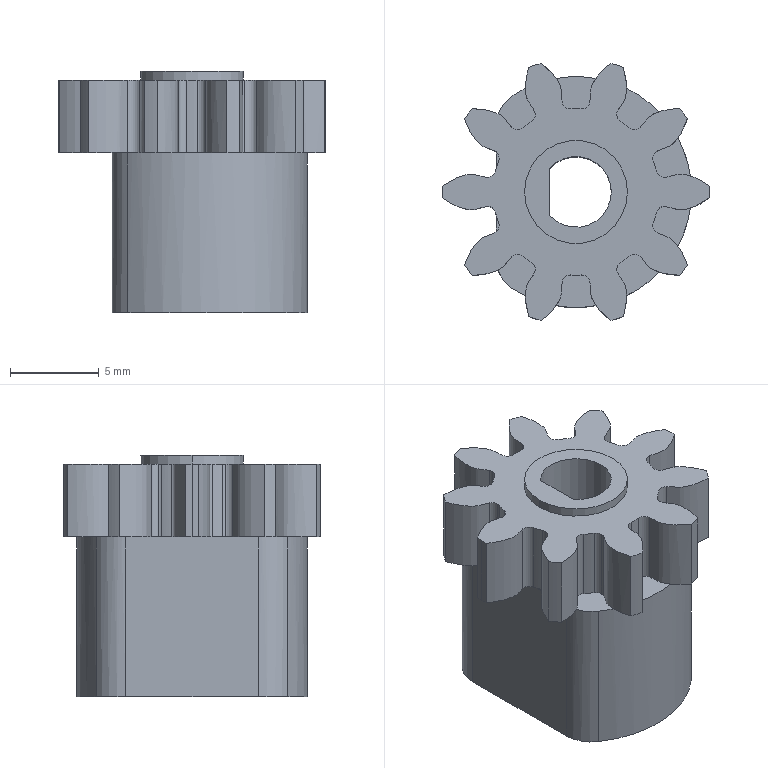Part | SolidWorks | features ICE 5, CirPattern 1, Extrusion 1, Fillet 1, RefAxis 1 | 1 solid | 97 faces | box 15 x 14.473 x 13.6 mm | volume 1407 mm3 | cylinder 52 | plane 25 | spline 20 | commonest cylinder face diameters 0.95 x24 15 x11 9.375 x10 4 x2 5.8 x2 13 x2